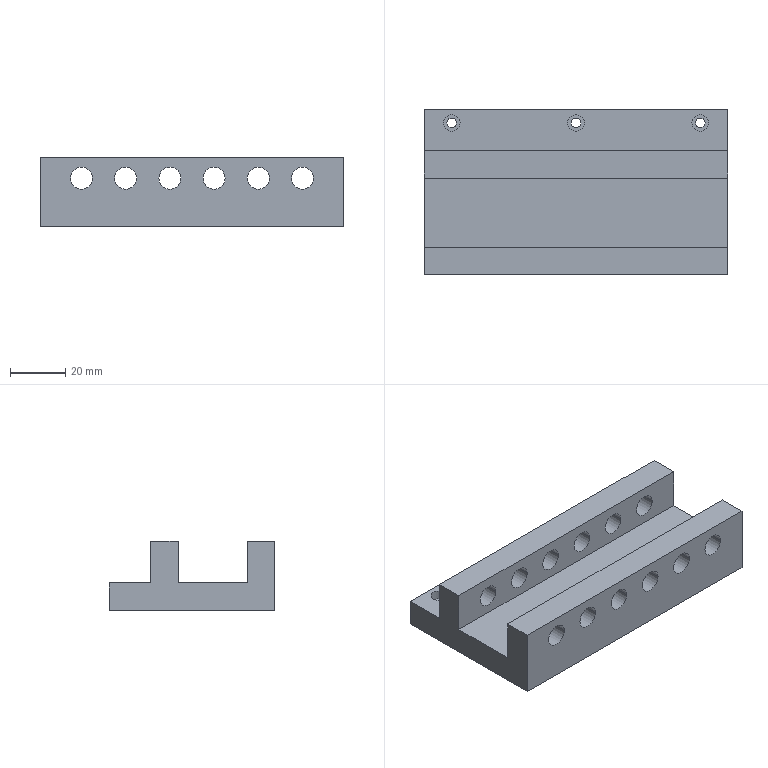Part | SolidWorks | features BaseBody 1 | 1 solid | 51 faces | box 110 x 60 x 25 mm | volume 92484 mm3 | cylinder 36 | plane 15 | commonest cylinder face diameters 8 x24 3.5 x6 6 x6